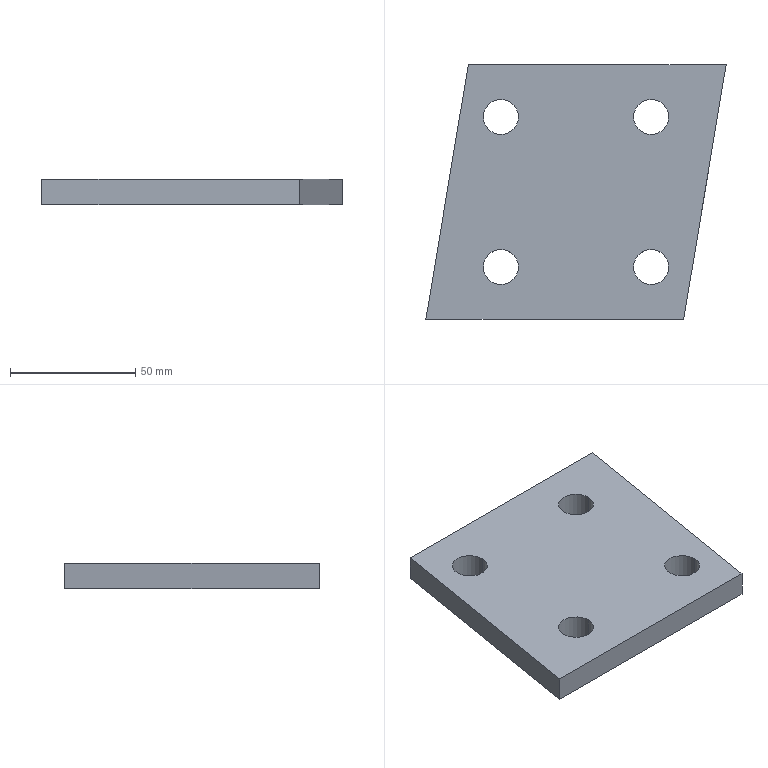Part | SolidWorks | features BaseBody 1 | 1 solid | 14 faces | box 120.015 x 101.6 x 10 mm | volume 98503 mm3 | cylinder 8 | plane 6 | commonest cylinder face diameters 14 x8
STEP:
#1=CARTESIAN_POINT('',(27.25,75.547,0.));
#2=VERTEX_POINT('',#1);
#3=CARTESIAN_POINT('',(13.25,75.547,0.));
#4=VERTEX_POINT('',#3);
#5=CARTESIAN_POINT('',(20.25,75.547,0.));
#6=DIRECTION('',(0.,0.,-1.));
#7=DIRECTION('',(1.,0.,0.));
#8=AXIS2_PLACEMENT_3D('',#5,#6,#7);
#9=CIRCLE('',#8,7.);
#10=EDGE_CURVE('',#2,#4,#9,.T.);
#11=ORIENTED_EDGE('',*,*,#10,.T.);
#12=CARTESIAN_POINT('',(13.25,75.547,10.));
#13=VERTEX_POINT('',#12);
#14=CARTESIAN_POINT('',(13.25,75.547,0.));
#15=DIRECTION('',(0.,0.,1.));
#16=VECTOR('',#15,1000.);
#17=LINE('',#14,#16);
#18=EDGE_CURVE('',#4,#13,#17,.T.);
#19=ORIENTED_EDGE('',*,*,#18,.T.);
#20=CARTESIAN_POINT('',(27.25,75.547,10.));
#21=VERTEX_POINT('',#20);
#22=CARTESIAN_POINT('',(20.25,75.547,10.));
#23=DIRECTION('',(0.,0.,-1.));
#24=DIRECTION('',(1.,0.,0.));
#25=AXIS2_PLACEMENT_3D('',#22,#23,#24);
#26=CIRCLE('',#25,7.);
#27=EDGE_CURVE('',#21,#13,#26,.T.);
#28=ORIENTED_EDGE('',*,*,#27,.F.);
#29=CARTESIAN_POINT('',(27.25,75.547,0.));
#30=DIRECTION('',(0.,0.,1.));
#31=VECTOR('',#30,1000.);
#32=LINE('',#29,#31);
#33=EDGE_CURVE('',#2,#21,#32,.T.);
#34=ORIENTED_EDGE('',*,*,#33,.F.);
#35=EDGE_LOOP('',(#11,#19,#28,#34));
#36=FACE_OUTER_BOUND('',#35,.T.);
#37=CARTESIAN_POINT('',(20.25,75.547,0.));
#38=DIRECTION('',(0.,0.,1.));
#39=DIRECTION('',(1.,0.,0.));
#40=AXIS2_PLACEMENT_3D('',#37,#38,#39);
#41=CYLINDRICAL_SURFACE('',#40,7.);
#42=ADVANCED_FACE('',(#36),#41,.F.);
#43=CARTESIAN_POINT('',(87.25,75.547,0.));
#44=VERTEX_POINT('',#43);
#45=CARTESIAN_POINT('',(73.25,75.547,0.));
#46=VERTEX_POINT('',#45);
#47=CARTESIAN_POINT('',(80.25,75.547,0.));
#48=DIRECTION('',(0.,0.,-1.));
#49=DIRECTION('',(1.,0.,0.));
#50=AXIS2_PLACEMENT_3D('',#47,#48,#49);
#51=CIRCLE('',#50,7.);
#52=EDGE_CURVE('',#44,#46,#51,.T.);
#53=ORIENTED_EDGE('',*,*,#52,.T.);
#54=CARTESIAN_POINT('',(73.25,75.547,10.));
#55=VERTEX_POINT('',#54);
#56=CARTESIAN_POINT('',(73.25,75.547,0.));
#57=DIRECTION('',(0.,0.,1.));
#58=VECTOR('',#57,1000.);
#59=LINE('',#56,#58);
#60=EDGE_CURVE('',#46,#55,#59,.T.);
#61=ORIENTED_EDGE('',*,*,#60,.T.);
#62=CARTESIAN_POINT('',(87.25,75.547,10.));
#63=VERTEX_POINT('',#62);
#64=CARTESIAN_POINT('',(80.25,75.547,10.));
#65=DIRECTION('',(0.,0.,-1.));
#66=DIRECTION('',(1.,0.,0.));
#67=AXIS2_PLACEMENT_3D('',#64,#65,#66);
#68=CIRCLE('',#67,7.);
#69=EDGE_CURVE('',#63,#55,#68,.T.);
#70=ORIENTED_EDGE('',*,*,#69,.F.);
#71=CARTESIAN_POINT('',(87.25,75.547,0.));
#72=DIRECTION('',(0.,0.,1.));
#73=VECTOR('',#72,1000.);
#74=LINE('',#71,#73);
#75=EDGE_CURVE('',#44,#63,#74,.T.);
#76=ORIENTED_EDGE('',*,*,#75,.F.);
#77=EDGE_LOOP('',(#53,#61,#70,#76));
#78=FACE_OUTER_BOUND('',#77,.T.);
#79=CARTESIAN_POINT('',(80.25,75.547,0.));
#80=DIRECTION('',(0.,0.,1.));
#81=DIRECTION('',(1.,0.,0.));
#82=AXIS2_PLACEMENT_3D('',#79,#80,#81);
#83=CYLINDRICAL_SURFACE('',#82,7.);
#84=ADVANCED_FACE('',(#78),#83,.F.);
#85=CARTESIAN_POINT('',(27.25,15.547,0.));
#86=VERTEX_POINT('',#85);
#87=CARTESIAN_POINT('',(13.25,15.547,0.));
#88=VERTEX_POINT('',#87);
#89=CARTESIAN_POINT('',(20.25,15.547,0.));
#90=DIRECTION('',(0.,0.,-1.));
#91=DIRECTION('',(1.,0.,0.));
#92=AXIS2_PLACEMENT_3D('',#89,#90,#91);
#93=CIRCLE('',#92,7.);
#94=EDGE_CURVE('',#86,#88,#93,.T.);
#95=ORIENTED_EDGE('',*,*,#94,.T.);
#96=CARTESIAN_POINT('',(13.25,15.547,10.));
#97=VERTEX_POINT('',#96);
#98=CARTESIAN_POINT('',(13.25,15.547,0.));
#99=DIRECTION('',(0.,0.,1.));
#100=VECTOR('',#99,1000.);
#101=LINE('',#98,#100);
#102=EDGE_CURVE('',#88,#97,#101,.T.);
#103=ORIENTED_EDGE('',*,*,#102,.T.);
#104=CARTESIAN_POINT('',(27.25,15.547,10.));
#105=VERTEX_POINT('',#104);
#106=CARTESIAN_POINT('',(20.25,15.547,10.));
#107=DIRECTION('',(0.,0.,-1.));
#108=DIRECTION('',(1.,0.,0.));
#109=AXIS2_PLACEMENT_3D('',#106,#107,#108);
#110=CIRCLE('',#109,7.);
#111=EDGE_CURVE('',#105,#97,#110,.T.);
#112=ORIENTED_EDGE('',*,*,#111,.F.);
#113=CARTESIAN_POINT('',(27.25,15.547,0.));
#114=DIRECTION('',(0.,0.,1.));
#115=VECTOR('',#114,1000.);
#116=LINE('',#113,#115);
#117=EDGE_CURVE('',#86,#105,#116,.T.);
#118=ORIENTED_EDGE('',*,*,#117,.F.);
#119=EDGE_LOOP('',(#95,#103,#112,#118));
#120=FACE_OUTER_BOUND('',#119,.T.);
#121=CARTESIAN_POINT('',(20.25,15.547,0.));
#122=DIRECTION('',(0.,0.,1.));
#123=DIRECTION('',(1.,0.,0.));
#124=AXIS2_PLACEMENT_3D('',#121,#122,#123);
#125=CYLINDRICAL_SURFACE('',#124,7.);
#126=ADVANCED_FACE('',(#120),#125,.F.);
#127=CARTESIAN_POINT('',(87.25,15.547,0.));
#128=VERTEX_POINT('',#127);
#129=CARTESIAN_POINT('',(73.25,15.547,0.));
#130=VERTEX_POINT('',#129);
#131=CARTESIAN_POINT('',(80.25,15.547,0.));
#132=DIRECTION('',(0.,0.,-1.));
#133=DIRECTION('',(1.,0.,0.));
#134=AXIS2_PLACEMENT_3D('',#131,#132,#133);
#135=CIRCLE('',#134,7.);
#136=EDGE_CURVE('',#128,#130,#135,.T.);
#137=ORIENTED_EDGE('',*,*,#136,.T.);
#138=CARTESIAN_POINT('',(73.25,15.547,10.));
#139=VERTEX_POINT('',#138);
#140=CARTESIAN_POINT('',(73.25,15.547,0.));
#141=DIRECTION('',(0.,0.,1.));
#142=VECTOR('',#141,1000.);
#143=LINE('',#140,#142);
#144=EDGE_CURVE('',#130,#139,#143,.T.);
#145=ORIENTED_EDGE('',*,*,#144,.T.);
#146=CARTESIAN_POINT('',(87.25,15.547,10.));
#147=VERTEX_POINT('',#146);
#148=CARTESIAN_POINT('',(80.25,15.547,10.));
#149=DIRECTION('',(0.,0.,-1.));
#150=DIRECTION('',(1.,0.,0.));
#151=AXIS2_PLACEMENT_3D('',#148,#149,#150);
#152=CIRCLE('',#151,7.);
#153=EDGE_CURVE('',#147,#139,#152,.T.);
#154=ORIENTED_EDGE('',*,*,#153,.F.);
#155=CARTESIAN_POINT('',(87.25,15.547,0.));
#156=DIRECTION('',(0.,0.,1.));
#157=VECTOR('',#156,1000.);
#158=LINE('',#155,#157);
#159=EDGE_CURVE('',#128,#147,#158,.T.);
#160=ORIENTED_EDGE('',*,*,#159,.F.);
#161=EDGE_LOOP('',(#137,#145,#154,#160));
#162=FACE_OUTER_BOUND('',#161,.T.);
#163=CARTESIAN_POINT('',(80.25,15.547,0.));
#164=DIRECTION('',(0.,0.,1.));
#165=DIRECTION('',(1.,0.,0.));
#166=AXIS2_PLACEMENT_3D('',#163,#164,#165);
#167=CYLINDRICAL_SURFACE('',#166,7.);
#168=ADVANCED_FACE('',(#162),#167,.F.);
#169=ORIENTED_EDGE('',*,*,#10,.F.);
#170=CARTESIAN_POINT('',(20.25,75.547,0.));
#171=DIRECTION('',(0.,0.,-1.));
#172=DIRECTION('',(1.,0.,0.));
#173=AXIS2_PLACEMENT_3D('',#170,#171,#172);
#174=CIRCLE('',#173,7.);
#175=EDGE_CURVE('',#4,#2,#174,.T.);
#176=ORIENTED_EDGE('',*,*,#175,.F.);
#177=EDGE_LOOP('',(#169,#176));
#178=FACE_BOUND('',#177,.T.);
#179=ORIENTED_EDGE('',*,*,#52,.F.);
#180=CARTESIAN_POINT('',(80.25,75.547,0.));
#181=DIRECTION('',(0.,0.,-1.));
#182=DIRECTION('',(1.,0.,0.));
#183=AXIS2_PLACEMENT_3D('',#180,#181,#182);
#184=CIRCLE('',#183,7.);
#185=EDGE_CURVE('',#46,#44,#184,.T.);
#186=ORIENTED_EDGE('',*,*,#185,.F.);
#187=EDGE_LOOP('',(#179,#186));
#188=FACE_BOUND('',#187,.T.);
#189=ORIENTED_EDGE('',*,*,#94,.F.);
#190=CARTESIAN_POINT('',(20.25,15.547,0.));
#191=DIRECTION('',(0.,0.,-1.));
#192=DIRECTION('',(1.,0.,0.));
#193=AXIS2_PLACEMENT_3D('',#190,#191,#192);
#194=CIRCLE('',#193,7.);
#195=EDGE_CURVE('',#88,#86,#194,.T.);
#196=ORIENTED_EDGE('',*,*,#195,.F.);
#197=EDGE_LOOP('',(#189,#196));
#198=FACE_BOUND('',#197,.T.);
#199=ORIENTED_EDGE('',*,*,#136,.F.);
#200=CARTESIAN_POINT('',(80.25,15.547,0.));
#201=DIRECTION('',(0.,0.,-1.));
#202=DIRECTION('',(1.,0.,0.));
#203=AXIS2_PLACEMENT_3D('',#200,#201,#202);
#204=CIRCLE('',#203,7.);
#205=EDGE_CURVE('',#130,#128,#204,.T.);
#206=ORIENTED_EDGE('',*,*,#205,.F.);
#207=EDGE_LOOP('',(#199,#206));
#208=FACE_BOUND('',#207,.T.);
#209=CARTESIAN_POINT('',(110.257,96.347,0.));
#210=VERTEX_POINT('',#209);
#211=CARTESIAN_POINT('',(7.244,96.347,0.));
#212=VERTEX_POINT('',#211);
#213=CARTESIAN_POINT('',(50.25,96.347,0.));
#214=DIRECTION('',(-1.,0.,0.));
#215=VECTOR('',#214,1000.);
#216=LINE('',#213,#215);
#217=EDGE_CURVE('',#210,#212,#216,.T.);
#218=ORIENTED_EDGE('',*,*,#217,.F.);
#219=CARTESIAN_POINT('',(93.255,-5.253,0.));
#220=VERTEX_POINT('',#219);
#221=CARTESIAN_POINT('',(93.255,-5.253,0.));
#222=DIRECTION('',(0.165,0.9863,0.));
#223=VECTOR('',#222,1000.);
#224=LINE('',#221,#223);
#225=EDGE_CURVE('',#220,#210,#224,.T.);
#226=ORIENTED_EDGE('',*,*,#225,.F.);
#227=CARTESIAN_POINT('',(-9.758,-5.253,0.));
#228=VERTEX_POINT('',#227);
#229=CARTESIAN_POINT('',(50.25,-5.253,0.));
#230=DIRECTION('',(1.,0.,0.));
#231=VECTOR('',#230,1000.);
#232=LINE('',#229,#231);
#233=EDGE_CURVE('',#228,#220,#232,.T.);
#234=ORIENTED_EDGE('',*,*,#233,.F.);
#235=CARTESIAN_POINT('',(7.244,96.347,0.));
#236=DIRECTION('',(-0.165,-0.9863,0.));
#237=VECTOR('',#236,1000.);
#238=LINE('',#235,#237);
#239=EDGE_CURVE('',#212,#228,#238,.T.);
#240=ORIENTED_EDGE('',*,*,#239,.F.);
#241=EDGE_LOOP('',(#218,#226,#234,#240));
#242=FACE_OUTER_BOUND('',#241,.T.);
#243=CARTESIAN_POINT('',(50.25,45.547,0.));
#244=DIRECTION('',(0.,0.,1.));
#245=DIRECTION('',(1.,0.,0.));
#246=AXIS2_PLACEMENT_3D('',#243,#244,#245);
#247=PLANE('',#246);
#248=ADVANCED_FACE('',(#178,#188,#198,#208,#242),#247,.F.);
#249=ORIENTED_EDGE('',*,*,#18,.F.);
#250=ORIENTED_EDGE('',*,*,#175,.T.);
#251=ORIENTED_EDGE('',*,*,#33,.T.);
#252=CARTESIAN_POINT('',(20.25,75.547,10.));
#253=DIRECTION('',(0.,0.,-1.));
#254=DIRECTION('',(1.,0.,0.));
#255=AXIS2_PLACEMENT_3D('',#252,#253,#254);
#256=CIRCLE('',#255,7.);
#257=EDGE_CURVE('',#13,#21,#256,.T.);
#258=ORIENTED_EDGE('',*,*,#257,.F.);
#259=EDGE_LOOP('',(#249,#250,#251,#258));
#260=FACE_OUTER_BOUND('',#259,.T.);
#261=CARTESIAN_POINT('',(20.25,75.547,0.));
#262=DIRECTION('',(0.,0.,1.));
#263=DIRECTION('',(1.,0.,0.));
#264=AXIS2_PLACEMENT_3D('',#261,#262,#263);
#265=CYLINDRICAL_SURFACE('',#264,7.);
#266=ADVANCED_FACE('',(#260),#265,.F.);
#267=ORIENTED_EDGE('',*,*,#60,.F.);
#268=ORIENTED_EDGE('',*,*,#185,.T.);
#269=ORIENTED_EDGE('',*,*,#75,.T.);
#270=CARTESIAN_POINT('',(80.25,75.547,10.));
#271=DIRECTION('',(0.,0.,-1.));
#272=DIRECTION('',(1.,0.,0.));
#273=AXIS2_PLACEMENT_3D('',#270,#271,#272);
#274=CIRCLE('',#273,7.);
#275=EDGE_CURVE('',#55,#63,#274,.T.);
#276=ORIENTED_EDGE('',*,*,#275,.F.);
#277=EDGE_LOOP('',(#267,#268,#269,#276));
#278=FACE_OUTER_BOUND('',#277,.T.);
#279=CARTESIAN_POINT('',(80.25,75.547,0.));
#280=DIRECTION('',(0.,0.,1.));
#281=DIRECTION('',(1.,0.,0.));
#282=AXIS2_PLACEMENT_3D('',#279,#280,#281);
#283=CYLINDRICAL_SURFACE('',#282,7.);
#284=ADVANCED_FACE('',(#278),#283,.F.);
#285=ORIENTED_EDGE('',*,*,#102,.F.);
#286=ORIENTED_EDGE('',*,*,#195,.T.);
#287=ORIENTED_EDGE('',*,*,#117,.T.);
#288=CARTESIAN_POINT('',(20.25,15.547,10.));
#289=DIRECTION('',(0.,0.,-1.));
#290=DIRECTION('',(1.,0.,0.));
#291=AXIS2_PLACEMENT_3D('',#288,#289,#290);
#292=CIRCLE('',#291,7.);
#293=EDGE_CURVE('',#97,#105,#292,.T.);
#294=ORIENTED_EDGE('',*,*,#293,.F.);
#295=EDGE_LOOP('',(#285,#286,#287,#294));
#296=FACE_OUTER_BOUND('',#295,.T.);
#297=CARTESIAN_POINT('',(20.25,15.547,0.));
#298=DIRECTION('',(0.,0.,1.));
#299=DIRECTION('',(1.,0.,0.));
#300=AXIS2_PLACEMENT_3D('',#297,#298,#299);
#301=CYLINDRICAL_SURFACE('',#300,7.);
#302=ADVANCED_FACE('',(#296),#301,.F.);
#303=ORIENTED_EDGE('',*,*,#144,.F.);
#304=ORIENTED_EDGE('',*,*,#205,.T.);
#305=ORIENTED_EDGE('',*,*,#159,.T.);
#306=CARTESIAN_POINT('',(80.25,15.547,10.));
#307=DIRECTION('',(0.,0.,-1.));
#308=DIRECTION('',(1.,0.,0.));
#309=AXIS2_PLACEMENT_3D('',#306,#307,#308);
#310=CIRCLE('',#309,7.);
#311=EDGE_CURVE('',#139,#147,#310,.T.);
#312=ORIENTED_EDGE('',*,*,#311,.F.);
#313=EDGE_LOOP('',(#303,#304,#305,#312));
#314=FACE_OUTER_BOUND('',#313,.T.);
#315=CARTESIAN_POINT('',(80.25,15.547,0.));
#316=DIRECTION('',(0.,0.,1.));
#317=DIRECTION('',(1.,0.,0.));
#318=AXIS2_PLACEMENT_3D('',#315,#316,#317);
#319=CYLINDRICAL_SURFACE('',#318,7.);
#320=ADVANCED_FACE('',(#314),#319,.F.);
#321=ORIENTED_EDGE('',*,*,#239,.T.);
#322=CARTESIAN_POINT('',(-9.758,-5.253,10.));
#323=VERTEX_POINT('',#322);
#324=CARTESIAN_POINT('',(-9.758,-5.253,0.));
#325=DIRECTION('',(0.,0.,1.));
#326=VECTOR('',#325,1000.);
#327=LINE('',#324,#326);
#328=EDGE_CURVE('',#228,#323,#327,.T.);
#329=ORIENTED_EDGE('',*,*,#328,.T.);
#330=CARTESIAN_POINT('',(7.244,96.347,10.));
#331=VERTEX_POINT('',#330);
#332=CARTESIAN_POINT('',(-9.758,-5.253,10.));
#333=DIRECTION('',(0.165,0.9863,0.));
#334=VECTOR('',#333,1000.);
#335=LINE('',#332,#334);
#336=EDGE_CURVE('',#323,#331,#335,.T.);
#337=ORIENTED_EDGE('',*,*,#336,.T.);
#338=CARTESIAN_POINT('',(7.244,96.347,0.));
#339=DIRECTION('',(0.,0.,-1.));
#340=VECTOR('',#339,1000.);
#341=LINE('',#338,#340);
#342=EDGE_CURVE('',#331,#212,#341,.T.);
#343=ORIENTED_EDGE('',*,*,#342,.T.);
#344=EDGE_LOOP('',(#321,#329,#337,#343));
#345=FACE_OUTER_BOUND('',#344,.T.);
#346=CARTESIAN_POINT('',(-9.758,-5.253,0.));
#347=DIRECTION('',(-0.9863,0.165,0.));
#348=DIRECTION('',(-0.165,-0.9863,0.));
#349=AXIS2_PLACEMENT_3D('',#346,#347,#348);
#350=PLANE('',#349);
#351=ADVANCED_FACE('',(#345),#350,.T.);
#352=ORIENTED_EDGE('',*,*,#217,.T.);
#353=ORIENTED_EDGE('',*,*,#342,.F.);
#354=CARTESIAN_POINT('',(110.257,96.347,10.));
#355=VERTEX_POINT('',#354);
#356=CARTESIAN_POINT('',(7.244,96.347,10.));
#357=DIRECTION('',(1.,0.,0.));
#358=VECTOR('',#357,1000.);
#359=LINE('',#356,#358);
#360=EDGE_CURVE('',#331,#355,#359,.T.);
#361=ORIENTED_EDGE('',*,*,#360,.T.);
#362=CARTESIAN_POINT('',(110.257,96.347,0.));
#363=DIRECTION('',(0.,0.,-1.));
#364=VECTOR('',#363,1000.);
#365=LINE('',#362,#364);
#366=EDGE_CURVE('',#355,#210,#365,.T.);
#367=ORIENTED_EDGE('',*,*,#366,.T.);
#368=EDGE_LOOP('',(#352,#353,#361,#367));
#369=FACE_OUTER_BOUND('',#368,.T.);
#370=CARTESIAN_POINT('',(7.244,96.347,0.));
#371=DIRECTION('',(0.,1.,0.));
#372=DIRECTION('',(0.,0.,1.));
#373=AXIS2_PLACEMENT_3D('',#370,#371,#372);
#374=PLANE('',#373);
#375=ADVANCED_FACE('',(#369),#374,.T.);
#376=ORIENTED_EDGE('',*,*,#225,.T.);
#377=ORIENTED_EDGE('',*,*,#366,.F.);
#378=CARTESIAN_POINT('',(93.255,-5.253,10.));
#379=VERTEX_POINT('',#378);
#380=CARTESIAN_POINT('',(110.257,96.347,10.));
#381=DIRECTION('',(-0.165,-0.9863,0.));
#382=VECTOR('',#381,1000.);
#383=LINE('',#380,#382);
#384=EDGE_CURVE('',#355,#379,#383,.T.);
#385=ORIENTED_EDGE('',*,*,#384,.T.);
#386=CARTESIAN_POINT('',(93.255,-5.253,0.));
#387=DIRECTION('',(0.,0.,-1.));
#388=VECTOR('',#387,1000.);
#389=LINE('',#386,#388);
#390=EDGE_CURVE('',#379,#220,#389,.T.);
#391=ORIENTED_EDGE('',*,*,#390,.T.);
#392=EDGE_LOOP('',(#376,#377,#385,#391));
#393=FACE_OUTER_BOUND('',#392,.T.);
#394=CARTESIAN_POINT('',(110.257,96.347,0.));
#395=DIRECTION('',(0.9863,-0.165,0.));
#396=DIRECTION('',(0.165,0.9863,0.));
#397=AXIS2_PLACEMENT_3D('',#394,#395,#396);
#398=PLANE('',#397);
#399=ADVANCED_FACE('',(#393),#398,.T.);
#400=ORIENTED_EDGE('',*,*,#233,.T.);
#401=ORIENTED_EDGE('',*,*,#390,.F.);
#402=CARTESIAN_POINT('',(93.255,-5.253,10.));
#403=DIRECTION('',(-1.,0.,0.));
#404=VECTOR('',#403,1000.);
#405=LINE('',#402,#404);
#406=EDGE_CURVE('',#379,#323,#405,.T.);
#407=ORIENTED_EDGE('',*,*,#406,.T.);
#408=ORIENTED_EDGE('',*,*,#328,.F.);
#409=EDGE_LOOP('',(#400,#401,#407,#408));
#410=FACE_OUTER_BOUND('',#409,.T.);
#411=CARTESIAN_POINT('',(93.255,-5.253,0.));
#412=DIRECTION('',(0.,-1.,0.));
#413=DIRECTION('',(0.,0.,-1.));
#414=AXIS2_PLACEMENT_3D('',#411,#412,#413);
#415=PLANE('',#414);
#416=ADVANCED_FACE('',(#410),#415,.T.);
#417=ORIENTED_EDGE('',*,*,#27,.T.);
#418=ORIENTED_EDGE('',*,*,#257,.T.);
#419=EDGE_LOOP('',(#417,#418));
#420=FACE_BOUND('',#419,.T.);
#421=ORIENTED_EDGE('',*,*,#69,.T.);
#422=ORIENTED_EDGE('',*,*,#275,.T.);
#423=EDGE_LOOP('',(#421,#422));
#424=FACE_BOUND('',#423,.T.);
#425=ORIENTED_EDGE('',*,*,#111,.T.);
#426=ORIENTED_EDGE('',*,*,#293,.T.);
#427=EDGE_LOOP('',(#425,#426));
#428=FACE_BOUND('',#427,.T.);
#429=ORIENTED_EDGE('',*,*,#153,.T.);
#430=ORIENTED_EDGE('',*,*,#311,.T.);
#431=EDGE_LOOP('',(#429,#430));
#432=FACE_BOUND('',#431,.T.);
#433=ORIENTED_EDGE('',*,*,#406,.F.);
#434=ORIENTED_EDGE('',*,*,#384,.F.);
#435=ORIENTED_EDGE('',*,*,#360,.F.);
#436=ORIENTED_EDGE('',*,*,#336,.F.);
#437=EDGE_LOOP('',(#433,#434,#435,#436));
#438=FACE_OUTER_BOUND('',#437,.T.);
#439=CARTESIAN_POINT('',(50.25,45.547,10.));
#440=DIRECTION('',(0.,0.,1.));
#441=DIRECTION('',(1.,0.,0.));
#442=AXIS2_PLACEMENT_3D('',#439,#440,#441);
#443=PLANE('',#442);
#444=ADVANCED_FACE('',(#420,#424,#428,#432,#438),#443,.T.);
#445=CLOSED_SHELL('',(#42,#84,#126,#168,#248,#266,#284,#302,#320,#351,#375,#399,#416,#444));
#446=MANIFOLD_SOLID_BREP('',#445);
#447=CARTESIAN_POINT('',(0.,0.,0.));
#448=DIRECTION('',(0.,0.,1.));
#449=DIRECTION('',(1.,0.,0.));
#450=AXIS2_PLACEMENT_3D('',#447,#448,#449);
#451=(LENGTH_UNIT()NAMED_UNIT(*)SI_UNIT(.MILLI.,.METRE.));
#452=UNCERTAINTY_MEASURE_WITH_UNIT(LENGTH_MEASURE(0.00001),#451,'','');
#453=(NAMED_UNIT(*)PLANE_ANGLE_UNIT()SI_UNIT($,.RADIAN.));
#454=(NAMED_UNIT(*)SI_UNIT($,.STERADIAN.)SOLID_ANGLE_UNIT());
#455=(GEOMETRIC_REPRESENTATION_CONTEXT(3)GLOBAL_UNCERTAINTY_ASSIGNED_CONTEXT((#452))GLOBAL_UNIT_ASSIGNED_CONTEXT((#451,#453,#454))REPRESENTATION_CONTEXT('',''));
#456=ADVANCED_BREP_SHAPE_REPRESENTATION('',(#446,#450),#455);